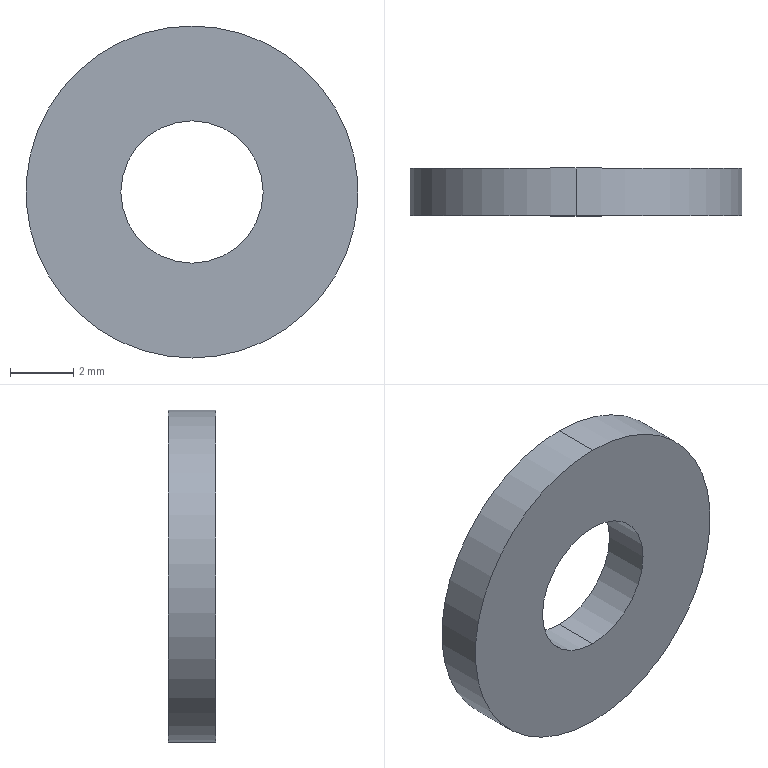Part | SolidWorks | features Extrusion 1 | 1 solid | 6 faces | box 10.5 x 1.5 x 10.5 mm | volume 106.029 mm3 | cylinder 4 | plane 2 | commonest cylinder face diameters 4.5 x2 10.5 x2
STEP:
#1=CARTESIAN_POINT('',(0.,1.5,-2.25));
#2=VERTEX_POINT('',#1);
#3=CARTESIAN_POINT('',(0.,1.5,2.25));
#4=VERTEX_POINT('',#3);
#5=CARTESIAN_POINT('',(0.,1.5,0.));
#6=DIRECTION('',(0.,1.,0.));
#7=DIRECTION('',(0.,0.,1.));
#8=AXIS2_PLACEMENT_3D('',#5,#6,#7);
#9=CIRCLE('',#8,2.25);
#10=EDGE_CURVE('',#2,#4,#9,.T.);
#11=ORIENTED_EDGE('',*,*,#10,.T.);
#12=CARTESIAN_POINT('',(0.,0.,2.25));
#13=VERTEX_POINT('',#12);
#14=CARTESIAN_POINT('',(0.,1.5,2.25));
#15=DIRECTION('',(0.,-1.,0.));
#16=VECTOR('',#15,1000.);
#17=LINE('',#14,#16);
#18=EDGE_CURVE('',#4,#13,#17,.T.);
#19=ORIENTED_EDGE('',*,*,#18,.T.);
#20=CARTESIAN_POINT('',(0.,0.,-2.25));
#21=VERTEX_POINT('',#20);
#22=CARTESIAN_POINT('',(0.,0.,0.));
#23=DIRECTION('',(0.,1.,0.));
#24=DIRECTION('',(0.,0.,1.));
#25=AXIS2_PLACEMENT_3D('',#22,#23,#24);
#26=CIRCLE('',#25,2.25);
#27=EDGE_CURVE('',#21,#13,#26,.T.);
#28=ORIENTED_EDGE('',*,*,#27,.F.);
#29=CARTESIAN_POINT('',(0.,1.5,-2.25));
#30=DIRECTION('',(0.,-1.,0.));
#31=VECTOR('',#30,1000.);
#32=LINE('',#29,#31);
#33=EDGE_CURVE('',#2,#21,#32,.T.);
#34=ORIENTED_EDGE('',*,*,#33,.F.);
#35=EDGE_LOOP('',(#11,#19,#28,#34));
#36=FACE_OUTER_BOUND('',#35,.T.);
#37=CARTESIAN_POINT('',(0.,1.5,0.));
#38=DIRECTION('',(0.,-1.,0.));
#39=DIRECTION('',(0.,0.,-1.));
#40=AXIS2_PLACEMENT_3D('',#37,#38,#39);
#41=CYLINDRICAL_SURFACE('',#40,2.25);
#42=ADVANCED_FACE('',(#36),#41,.F.);
#43=CARTESIAN_POINT('',(0.,1.5,5.25));
#44=VERTEX_POINT('',#43);
#45=CARTESIAN_POINT('',(0.,1.5,-5.25));
#46=VERTEX_POINT('',#45);
#47=CARTESIAN_POINT('',(0.,1.5,0.));
#48=DIRECTION('',(0.,1.,0.));
#49=DIRECTION('',(0.,0.,1.));
#50=AXIS2_PLACEMENT_3D('',#47,#48,#49);
#51=CIRCLE('',#50,5.25);
#52=EDGE_CURVE('',#44,#46,#51,.T.);
#53=ORIENTED_EDGE('',*,*,#52,.F.);
#54=CARTESIAN_POINT('',(0.,0.,5.25));
#55=VERTEX_POINT('',#54);
#56=CARTESIAN_POINT('',(0.,1.5,5.25));
#57=DIRECTION('',(0.,-1.,0.));
#58=VECTOR('',#57,1000.);
#59=LINE('',#56,#58);
#60=EDGE_CURVE('',#44,#55,#59,.T.);
#61=ORIENTED_EDGE('',*,*,#60,.T.);
#62=CARTESIAN_POINT('',(0.,0.,-5.25));
#63=VERTEX_POINT('',#62);
#64=CARTESIAN_POINT('',(0.,0.,0.));
#65=DIRECTION('',(0.,1.,0.));
#66=DIRECTION('',(0.,0.,1.));
#67=AXIS2_PLACEMENT_3D('',#64,#65,#66);
#68=CIRCLE('',#67,5.25);
#69=EDGE_CURVE('',#55,#63,#68,.T.);
#70=ORIENTED_EDGE('',*,*,#69,.T.);
#71=CARTESIAN_POINT('',(0.,1.5,-5.25));
#72=DIRECTION('',(0.,-1.,0.));
#73=VECTOR('',#72,1000.);
#74=LINE('',#71,#73);
#75=EDGE_CURVE('',#46,#63,#74,.T.);
#76=ORIENTED_EDGE('',*,*,#75,.F.);
#77=EDGE_LOOP('',(#53,#61,#70,#76));
#78=FACE_OUTER_BOUND('',#77,.T.);
#79=CARTESIAN_POINT('',(0.,1.5,0.));
#80=DIRECTION('',(0.,-1.,0.));
#81=DIRECTION('',(0.,0.,-1.));
#82=AXIS2_PLACEMENT_3D('',#79,#80,#81);
#83=CYLINDRICAL_SURFACE('',#82,5.25);
#84=ADVANCED_FACE('',(#78),#83,.T.);
#85=CARTESIAN_POINT('',(0.,1.5,0.));
#86=DIRECTION('',(0.,1.,0.));
#87=DIRECTION('',(0.,0.,1.));
#88=AXIS2_PLACEMENT_3D('',#85,#86,#87);
#89=CIRCLE('',#88,5.25);
#90=EDGE_CURVE('',#46,#44,#89,.T.);
#91=ORIENTED_EDGE('',*,*,#90,.T.);
#92=ORIENTED_EDGE('',*,*,#52,.T.);
#93=EDGE_LOOP('',(#91,#92));
#94=FACE_OUTER_BOUND('',#93,.T.);
#95=ORIENTED_EDGE('',*,*,#10,.F.);
#96=CARTESIAN_POINT('',(0.,1.5,0.));
#97=DIRECTION('',(0.,1.,0.));
#98=DIRECTION('',(0.,0.,1.));
#99=AXIS2_PLACEMENT_3D('',#96,#97,#98);
#100=CIRCLE('',#99,2.25);
#101=EDGE_CURVE('',#4,#2,#100,.T.);
#102=ORIENTED_EDGE('',*,*,#101,.F.);
#103=EDGE_LOOP('',(#95,#102));
#104=FACE_BOUND('',#103,.T.);
#105=CARTESIAN_POINT('',(0.,1.5,0.));
#106=DIRECTION('',(0.,1.,0.));
#107=DIRECTION('',(0.,0.,1.));
#108=AXIS2_PLACEMENT_3D('',#105,#106,#107);
#109=PLANE('',#108);
#110=ADVANCED_FACE('',(#94,#104),#109,.T.);
#111=CARTESIAN_POINT('',(0.,0.,0.));
#112=DIRECTION('',(0.,1.,0.));
#113=DIRECTION('',(0.,0.,1.));
#114=AXIS2_PLACEMENT_3D('',#111,#112,#113);
#115=CIRCLE('',#114,5.25);
#116=EDGE_CURVE('',#63,#55,#115,.T.);
#117=ORIENTED_EDGE('',*,*,#116,.F.);
#118=ORIENTED_EDGE('',*,*,#69,.F.);
#119=EDGE_LOOP('',(#117,#118));
#120=FACE_OUTER_BOUND('',#119,.T.);
#121=ORIENTED_EDGE('',*,*,#27,.T.);
#122=CARTESIAN_POINT('',(0.,0.,0.));
#123=DIRECTION('',(0.,1.,0.));
#124=DIRECTION('',(0.,0.,1.));
#125=AXIS2_PLACEMENT_3D('',#122,#123,#124);
#126=CIRCLE('',#125,2.25);
#127=EDGE_CURVE('',#13,#21,#126,.T.);
#128=ORIENTED_EDGE('',*,*,#127,.T.);
#129=EDGE_LOOP('',(#121,#128));
#130=FACE_BOUND('',#129,.T.);
#131=CARTESIAN_POINT('',(0.,0.,0.));
#132=DIRECTION('',(0.,1.,0.));
#133=DIRECTION('',(0.,0.,1.));
#134=AXIS2_PLACEMENT_3D('',#131,#132,#133);
#135=PLANE('',#134);
#136=ADVANCED_FACE('',(#120,#130),#135,.F.);
#137=ORIENTED_EDGE('',*,*,#60,.F.);
#138=ORIENTED_EDGE('',*,*,#90,.F.);
#139=ORIENTED_EDGE('',*,*,#75,.T.);
#140=ORIENTED_EDGE('',*,*,#116,.T.);
#141=EDGE_LOOP('',(#137,#138,#139,#140));
#142=FACE_OUTER_BOUND('',#141,.T.);
#143=CARTESIAN_POINT('',(0.,1.5,0.));
#144=DIRECTION('',(0.,-1.,0.));
#145=DIRECTION('',(0.,0.,-1.));
#146=AXIS2_PLACEMENT_3D('',#143,#144,#145);
#147=CYLINDRICAL_SURFACE('',#146,5.25);
#148=ADVANCED_FACE('',(#142),#147,.T.);
#149=ORIENTED_EDGE('',*,*,#18,.F.);
#150=ORIENTED_EDGE('',*,*,#101,.T.);
#151=ORIENTED_EDGE('',*,*,#33,.T.);
#152=ORIENTED_EDGE('',*,*,#127,.F.);
#153=EDGE_LOOP('',(#149,#150,#151,#152));
#154=FACE_OUTER_BOUND('',#153,.T.);
#155=CARTESIAN_POINT('',(0.,1.5,0.));
#156=DIRECTION('',(0.,-1.,0.));
#157=DIRECTION('',(0.,0.,-1.));
#158=AXIS2_PLACEMENT_3D('',#155,#156,#157);
#159=CYLINDRICAL_SURFACE('',#158,2.25);
#160=ADVANCED_FACE('',(#154),#159,.F.);
#161=CLOSED_SHELL('',(#42,#84,#110,#136,#148,#160));
#162=MANIFOLD_SOLID_BREP('',#161);
#163=CARTESIAN_POINT('',(0.,0.,0.));
#164=DIRECTION('',(0.,0.,1.));
#165=DIRECTION('',(1.,0.,0.));
#166=AXIS2_PLACEMENT_3D('',#163,#164,#165);
#167=(LENGTH_UNIT()NAMED_UNIT(*)SI_UNIT(.MILLI.,.METRE.));
#168=UNCERTAINTY_MEASURE_WITH_UNIT(LENGTH_MEASURE(0.00001),#167,'','');
#169=(NAMED_UNIT(*)PLANE_ANGLE_UNIT()SI_UNIT($,.RADIAN.));
#170=(NAMED_UNIT(*)SI_UNIT($,.STERADIAN.)SOLID_ANGLE_UNIT());
#171=(GEOMETRIC_REPRESENTATION_CONTEXT(3)GLOBAL_UNCERTAINTY_ASSIGNED_CONTEXT((#168))GLOBAL_UNIT_ASSIGNED_CONTEXT((#167,#169,#170))REPRESENTATION_CONTEXT('',''));
#172=ADVANCED_BREP_SHAPE_REPRESENTATION('',(#162,#166),#171);